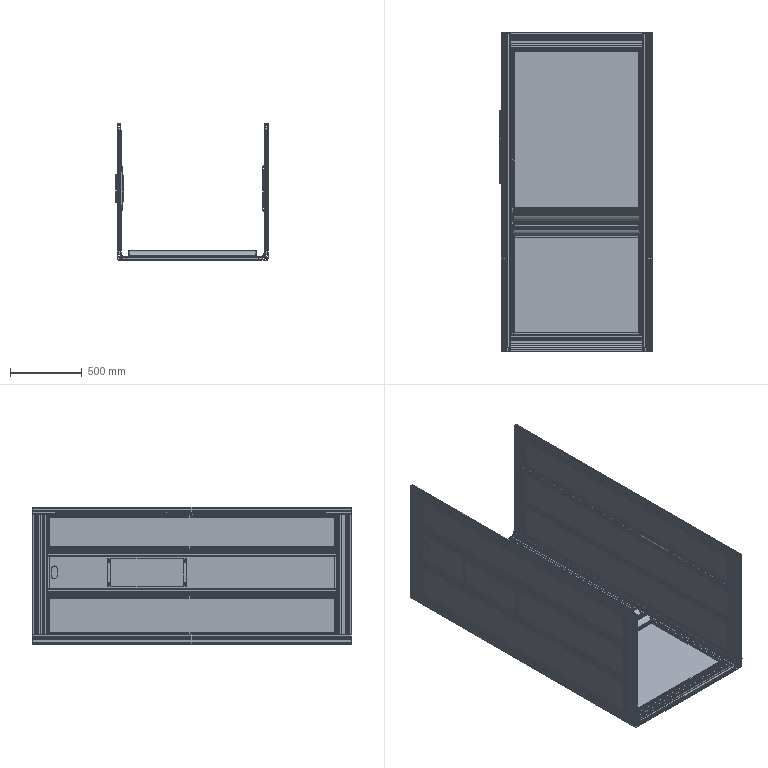Part | 152 solids | 5385 faces | volume 159628521 mm3 | plane 3496 | cylinder 1889 | commonest cylinder face diameters 1.1 x240 3.6 x204 8.5 x204 5.8 x198 0.4 x131 0.6 x112